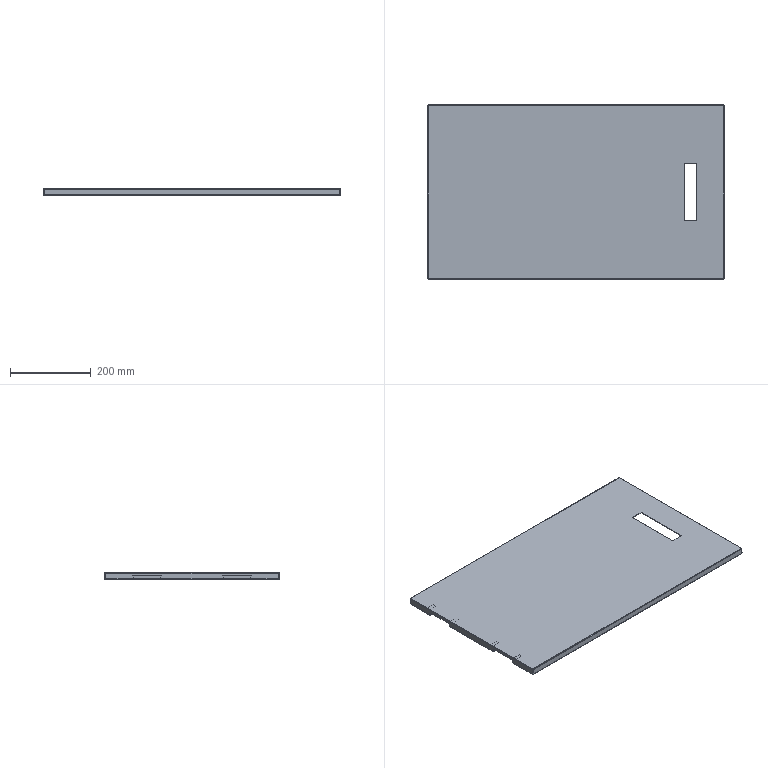Part | NX | features BREP 3 | 3 solids | 178 faces | box 736 x 432 x 16.5 mm | volume 552080 mm3 | plane 114 | cylinder 48 | spline 16 | commonest cylinder face diameters 0.02 x18 3.02 x18 3.2 x12